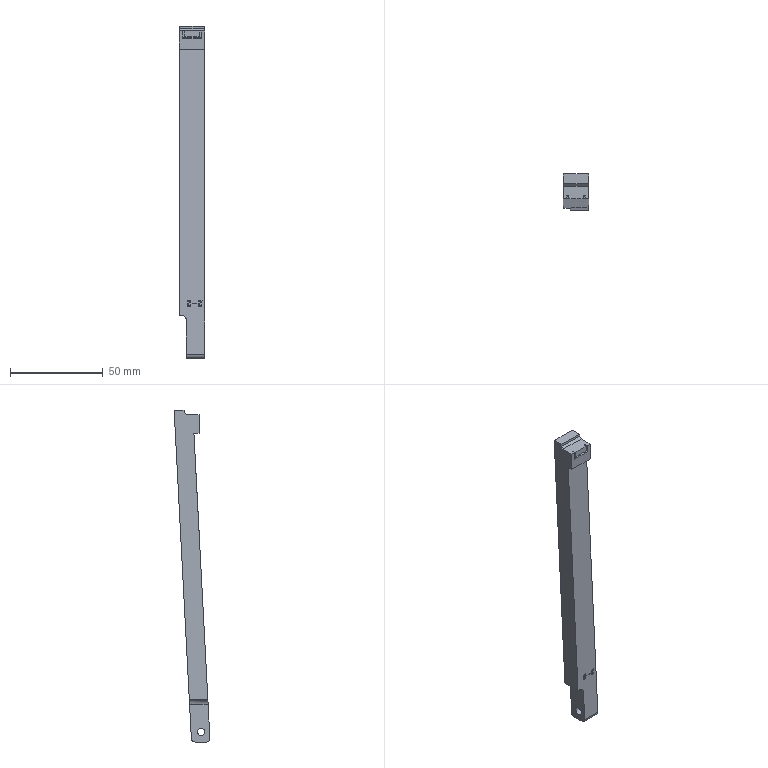Part | STEP file | solid 138 | 1 solid | 45 faces | box 14 x 19.289 x 179.041 mm | volume 24279 mm3 | plane 31 | cylinder 8 | other 4 | cone 1 | torus 1 | commonest cylinder face diameters 4 x3 4377 x2 6 x1 4372 x1 4375 x1